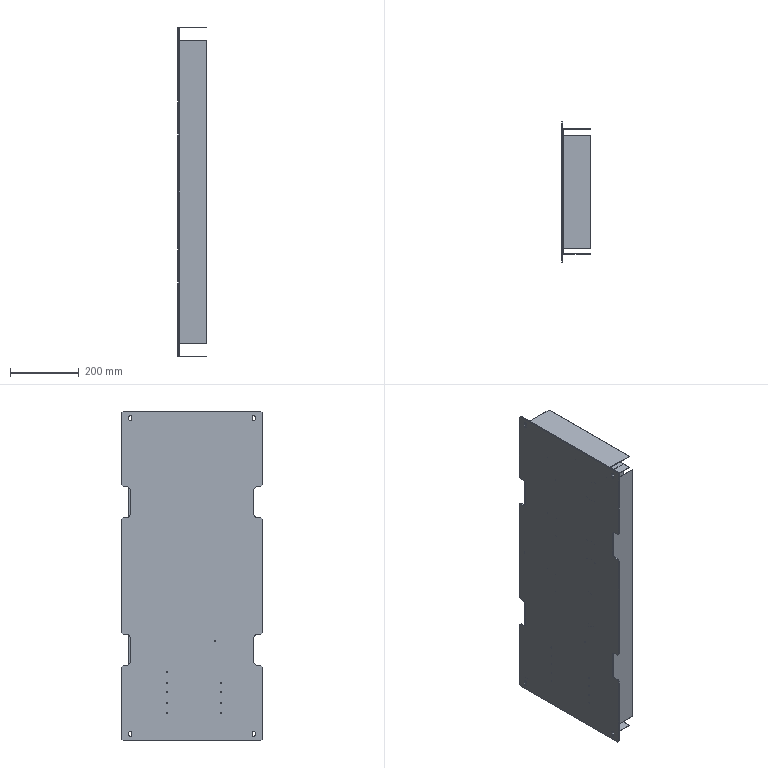Part | SolidWorks | 15 solids | 556 faces | box 83 x 410 x 960 mm | volume 1885959 mm3 | plane 280 | cylinder 276 | commonest cylinder face diameters 5.352 x56 4.5 x44 1.473 x40 2.5 x36 3.3 x20 4.2 x20